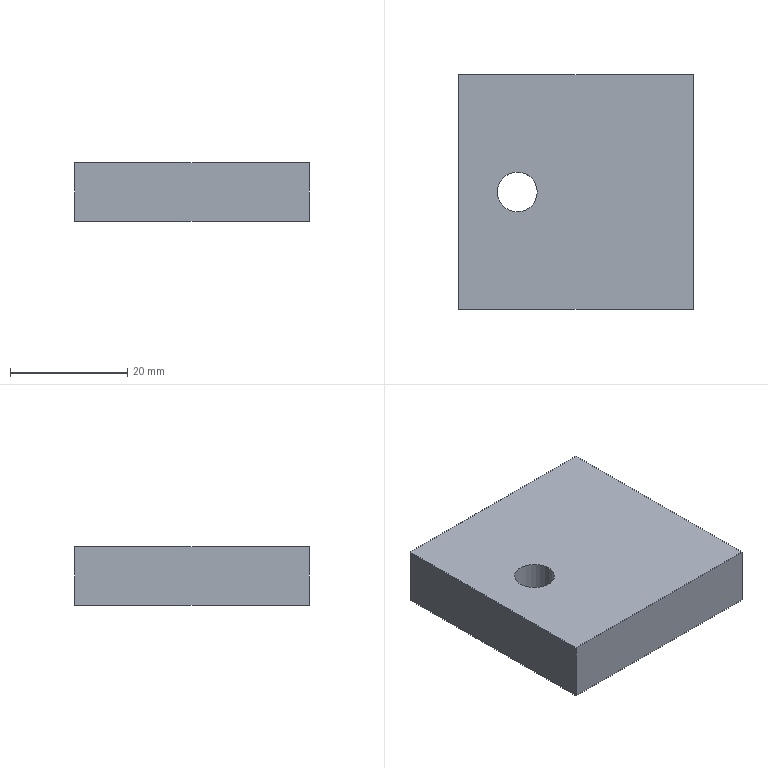Part | SolidWorks | features Extrusion 1, HoleWzd 1 | 1 solid | 8 faces | box 40 x 40 x 10 mm | volume 15637 mm3 | plane 6 | cylinder 2 | commonest cylinder face diameters 6.8 x2
STEP:
#1=CARTESIAN_POINT('',(-13.4,0.,-5.));
#2=VERTEX_POINT('',#1);
#3=CARTESIAN_POINT('',(-6.6,0.,-5.));
#4=VERTEX_POINT('',#3);
#5=CARTESIAN_POINT('',(-10.,0.,-5.));
#6=DIRECTION('',(0.,0.,1.));
#7=DIRECTION('',(1.,0.,0.));
#8=AXIS2_PLACEMENT_3D('',#5,#6,#7);
#9=CIRCLE('',#8,3.4);
#10=EDGE_CURVE('',#2,#4,#9,.T.);
#11=ORIENTED_EDGE('',*,*,#10,.F.);
#12=CARTESIAN_POINT('',(-13.4,0.,5.));
#13=VERTEX_POINT('',#12);
#14=CARTESIAN_POINT('',(-13.4,0.,5.));
#15=DIRECTION('',(0.,0.,1.));
#16=VECTOR('',#15,1000.);
#17=LINE('',#14,#16);
#18=EDGE_CURVE('',#2,#13,#17,.T.);
#19=ORIENTED_EDGE('',*,*,#18,.T.);
#20=CARTESIAN_POINT('',(-6.6,0.,5.));
#21=VERTEX_POINT('',#20);
#22=CARTESIAN_POINT('',(-10.,0.,5.));
#23=DIRECTION('',(0.,0.,1.));
#24=DIRECTION('',(1.,0.,0.));
#25=AXIS2_PLACEMENT_3D('',#22,#23,#24);
#26=CIRCLE('',#25,3.4);
#27=EDGE_CURVE('',#13,#21,#26,.T.);
#28=ORIENTED_EDGE('',*,*,#27,.T.);
#29=CARTESIAN_POINT('',(-6.6,0.,5.));
#30=DIRECTION('',(0.,0.,1.));
#31=VECTOR('',#30,1000.);
#32=LINE('',#29,#31);
#33=EDGE_CURVE('',#4,#21,#32,.T.);
#34=ORIENTED_EDGE('',*,*,#33,.F.);
#35=EDGE_LOOP('',(#11,#19,#28,#34));
#36=FACE_OUTER_BOUND('',#35,.T.);
#37=CARTESIAN_POINT('',(-10.,0.,5.));
#38=DIRECTION('',(0.,0.,1.));
#39=DIRECTION('',(1.,0.,0.));
#40=AXIS2_PLACEMENT_3D('',#37,#38,#39);
#41=CYLINDRICAL_SURFACE('',#40,3.4);
#42=ADVANCED_FACE('',(#36),#41,.F.);
#43=CARTESIAN_POINT('',(20.,-20.,-5.));
#44=VERTEX_POINT('',#43);
#45=CARTESIAN_POINT('',(20.,20.,-5.));
#46=VERTEX_POINT('',#45);
#47=CARTESIAN_POINT('',(20.,-20.,-5.));
#48=DIRECTION('',(0.,1.,0.));
#49=VECTOR('',#48,1000.);
#50=LINE('',#47,#49);
#51=EDGE_CURVE('',#44,#46,#50,.T.);
#52=ORIENTED_EDGE('',*,*,#51,.T.);
#53=CARTESIAN_POINT('',(20.,20.,5.));
#54=VERTEX_POINT('',#53);
#55=CARTESIAN_POINT('',(20.,20.,5.));
#56=DIRECTION('',(0.,0.,-1.));
#57=VECTOR('',#56,1000.);
#58=LINE('',#55,#57);
#59=EDGE_CURVE('',#54,#46,#58,.T.);
#60=ORIENTED_EDGE('',*,*,#59,.F.);
#61=CARTESIAN_POINT('',(20.,-20.,5.));
#62=VERTEX_POINT('',#61);
#63=CARTESIAN_POINT('',(20.,-20.,5.));
#64=DIRECTION('',(0.,1.,0.));
#65=VECTOR('',#64,1000.);
#66=LINE('',#63,#65);
#67=EDGE_CURVE('',#62,#54,#66,.T.);
#68=ORIENTED_EDGE('',*,*,#67,.F.);
#69=CARTESIAN_POINT('',(20.,-20.,5.));
#70=DIRECTION('',(0.,0.,-1.));
#71=VECTOR('',#70,1000.);
#72=LINE('',#69,#71);
#73=EDGE_CURVE('',#62,#44,#72,.T.);
#74=ORIENTED_EDGE('',*,*,#73,.T.);
#75=EDGE_LOOP('',(#52,#60,#68,#74));
#76=FACE_OUTER_BOUND('',#75,.T.);
#77=CARTESIAN_POINT('',(20.,-20.,5.));
#78=DIRECTION('',(-1.,0.,0.));
#79=DIRECTION('',(0.,0.,1.));
#80=AXIS2_PLACEMENT_3D('',#77,#78,#79);
#81=PLANE('',#80);
#82=ADVANCED_FACE('',(#76),#81,.F.);
#83=CARTESIAN_POINT('',(-20.,20.,-5.));
#84=VERTEX_POINT('',#83);
#85=CARTESIAN_POINT('',(-20.,20.,-5.));
#86=DIRECTION('',(-1.,0.,0.));
#87=VECTOR('',#86,1000.);
#88=LINE('',#85,#87);
#89=EDGE_CURVE('',#46,#84,#88,.T.);
#90=ORIENTED_EDGE('',*,*,#89,.T.);
#91=CARTESIAN_POINT('',(-20.,20.,5.));
#92=VERTEX_POINT('',#91);
#93=CARTESIAN_POINT('',(-20.,20.,5.));
#94=DIRECTION('',(0.,0.,-1.));
#95=VECTOR('',#94,1000.);
#96=LINE('',#93,#95);
#97=EDGE_CURVE('',#92,#84,#96,.T.);
#98=ORIENTED_EDGE('',*,*,#97,.F.);
#99=CARTESIAN_POINT('',(-20.,20.,5.));
#100=DIRECTION('',(-1.,0.,0.));
#101=VECTOR('',#100,1000.);
#102=LINE('',#99,#101);
#103=EDGE_CURVE('',#54,#92,#102,.T.);
#104=ORIENTED_EDGE('',*,*,#103,.F.);
#105=ORIENTED_EDGE('',*,*,#59,.T.);
#106=EDGE_LOOP('',(#90,#98,#104,#105));
#107=FACE_OUTER_BOUND('',#106,.T.);
#108=CARTESIAN_POINT('',(-20.,20.,5.));
#109=DIRECTION('',(0.,-1.,0.));
#110=DIRECTION('',(0.,0.,-1.));
#111=AXIS2_PLACEMENT_3D('',#108,#109,#110);
#112=PLANE('',#111);
#113=ADVANCED_FACE('',(#107),#112,.F.);
#114=CARTESIAN_POINT('',(-20.,-20.,-5.));
#115=VERTEX_POINT('',#114);
#116=CARTESIAN_POINT('',(-20.,-20.,-5.));
#117=DIRECTION('',(0.,-1.,0.));
#118=VECTOR('',#117,1000.);
#119=LINE('',#116,#118);
#120=EDGE_CURVE('',#84,#115,#119,.T.);
#121=ORIENTED_EDGE('',*,*,#120,.T.);
#122=CARTESIAN_POINT('',(-20.,-20.,5.));
#123=VERTEX_POINT('',#122);
#124=CARTESIAN_POINT('',(-20.,-20.,5.));
#125=DIRECTION('',(0.,0.,-1.));
#126=VECTOR('',#125,1000.);
#127=LINE('',#124,#126);
#128=EDGE_CURVE('',#123,#115,#127,.T.);
#129=ORIENTED_EDGE('',*,*,#128,.F.);
#130=CARTESIAN_POINT('',(-20.,-20.,5.));
#131=DIRECTION('',(0.,-1.,0.));
#132=VECTOR('',#131,1000.);
#133=LINE('',#130,#132);
#134=EDGE_CURVE('',#92,#123,#133,.T.);
#135=ORIENTED_EDGE('',*,*,#134,.F.);
#136=ORIENTED_EDGE('',*,*,#97,.T.);
#137=EDGE_LOOP('',(#121,#129,#135,#136));
#138=FACE_OUTER_BOUND('',#137,.T.);
#139=CARTESIAN_POINT('',(-20.,-20.,5.));
#140=DIRECTION('',(1.,0.,0.));
#141=DIRECTION('',(0.,0.,-1.));
#142=AXIS2_PLACEMENT_3D('',#139,#140,#141);
#143=PLANE('',#142);
#144=ADVANCED_FACE('',(#138),#143,.F.);
#145=CARTESIAN_POINT('',(-20.,-20.,-5.));
#146=DIRECTION('',(1.,0.,0.));
#147=VECTOR('',#146,1000.);
#148=LINE('',#145,#147);
#149=EDGE_CURVE('',#115,#44,#148,.T.);
#150=ORIENTED_EDGE('',*,*,#149,.T.);
#151=ORIENTED_EDGE('',*,*,#73,.F.);
#152=CARTESIAN_POINT('',(-20.,-20.,5.));
#153=DIRECTION('',(1.,0.,0.));
#154=VECTOR('',#153,1000.);
#155=LINE('',#152,#154);
#156=EDGE_CURVE('',#123,#62,#155,.T.);
#157=ORIENTED_EDGE('',*,*,#156,.F.);
#158=ORIENTED_EDGE('',*,*,#128,.T.);
#159=EDGE_LOOP('',(#150,#151,#157,#158));
#160=FACE_OUTER_BOUND('',#159,.T.);
#161=CARTESIAN_POINT('',(-20.,-20.,5.));
#162=DIRECTION('',(0.,1.,0.));
#163=DIRECTION('',(0.,0.,1.));
#164=AXIS2_PLACEMENT_3D('',#161,#162,#163);
#165=PLANE('',#164);
#166=ADVANCED_FACE('',(#160),#165,.F.);
#167=CARTESIAN_POINT('',(-10.,0.,5.));
#168=DIRECTION('',(0.,0.,1.));
#169=DIRECTION('',(1.,0.,0.));
#170=AXIS2_PLACEMENT_3D('',#167,#168,#169);
#171=CIRCLE('',#170,3.4);
#172=EDGE_CURVE('',#21,#13,#171,.T.);
#173=ORIENTED_EDGE('',*,*,#172,.F.);
#174=ORIENTED_EDGE('',*,*,#27,.F.);
#175=EDGE_LOOP('',(#173,#174));
#176=FACE_BOUND('',#175,.T.);
#177=ORIENTED_EDGE('',*,*,#67,.T.);
#178=ORIENTED_EDGE('',*,*,#103,.T.);
#179=ORIENTED_EDGE('',*,*,#134,.T.);
#180=ORIENTED_EDGE('',*,*,#156,.T.);
#181=EDGE_LOOP('',(#177,#178,#179,#180));
#182=FACE_OUTER_BOUND('',#181,.T.);
#183=CARTESIAN_POINT('',(0.,0.,5.));
#184=DIRECTION('',(0.,0.,-1.));
#185=DIRECTION('',(-1.,0.,0.));
#186=AXIS2_PLACEMENT_3D('',#183,#184,#185);
#187=PLANE('',#186);
#188=ADVANCED_FACE('',(#176,#182),#187,.F.);
#189=CARTESIAN_POINT('',(-10.,0.,-5.));
#190=DIRECTION('',(0.,0.,1.));
#191=DIRECTION('',(1.,0.,0.));
#192=AXIS2_PLACEMENT_3D('',#189,#190,#191);
#193=CIRCLE('',#192,3.4);
#194=EDGE_CURVE('',#4,#2,#193,.T.);
#195=ORIENTED_EDGE('',*,*,#194,.T.);
#196=ORIENTED_EDGE('',*,*,#10,.T.);
#197=EDGE_LOOP('',(#195,#196));
#198=FACE_BOUND('',#197,.T.);
#199=ORIENTED_EDGE('',*,*,#51,.F.);
#200=ORIENTED_EDGE('',*,*,#149,.F.);
#201=ORIENTED_EDGE('',*,*,#120,.F.);
#202=ORIENTED_EDGE('',*,*,#89,.F.);
#203=EDGE_LOOP('',(#199,#200,#201,#202));
#204=FACE_OUTER_BOUND('',#203,.T.);
#205=CARTESIAN_POINT('',(0.,0.,-5.));
#206=DIRECTION('',(0.,0.,-1.));
#207=DIRECTION('',(-1.,0.,0.));
#208=AXIS2_PLACEMENT_3D('',#205,#206,#207);
#209=PLANE('',#208);
#210=ADVANCED_FACE('',(#198,#204),#209,.T.);
#211=ORIENTED_EDGE('',*,*,#18,.F.);
#212=ORIENTED_EDGE('',*,*,#194,.F.);
#213=ORIENTED_EDGE('',*,*,#33,.T.);
#214=ORIENTED_EDGE('',*,*,#172,.T.);
#215=EDGE_LOOP('',(#211,#212,#213,#214));
#216=FACE_OUTER_BOUND('',#215,.T.);
#217=CARTESIAN_POINT('',(-10.,0.,5.));
#218=DIRECTION('',(0.,0.,1.));
#219=DIRECTION('',(1.,0.,0.));
#220=AXIS2_PLACEMENT_3D('',#217,#218,#219);
#221=CYLINDRICAL_SURFACE('',#220,3.4);
#222=ADVANCED_FACE('',(#216),#221,.F.);
#223=CLOSED_SHELL('',(#42,#82,#113,#144,#166,#188,#210,#222));
#224=MANIFOLD_SOLID_BREP('',#223);
#225=CARTESIAN_POINT('',(0.,0.,0.));
#226=DIRECTION('',(0.,0.,1.));
#227=DIRECTION('',(1.,0.,0.));
#228=AXIS2_PLACEMENT_3D('',#225,#226,#227);
#229=(LENGTH_UNIT()NAMED_UNIT(*)SI_UNIT(.MILLI.,.METRE.));
#230=UNCERTAINTY_MEASURE_WITH_UNIT(LENGTH_MEASURE(0.00001),#229,'','');
#231=(NAMED_UNIT(*)PLANE_ANGLE_UNIT()SI_UNIT($,.RADIAN.));
#232=(NAMED_UNIT(*)SI_UNIT($,.STERADIAN.)SOLID_ANGLE_UNIT());
#233=(GEOMETRIC_REPRESENTATION_CONTEXT(3)GLOBAL_UNCERTAINTY_ASSIGNED_CONTEXT((#230))GLOBAL_UNIT_ASSIGNED_CONTEXT((#229,#231,#232))REPRESENTATION_CONTEXT('',''));
#234=ADVANCED_BREP_SHAPE_REPRESENTATION('',(#224,#228),#233);